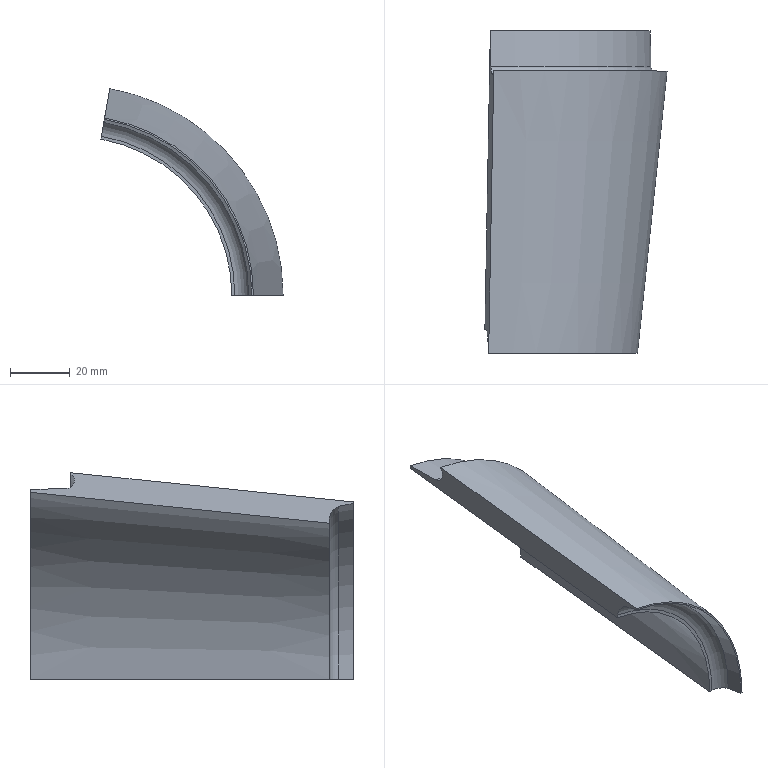Part | STEP file | rubber2 | 1 solid | 12 faces | box 60.803 x 107.596 x 68.922 mm | volume 62752 mm3 | plane 6 | cone 4 | torus 2
STEP:
#1=CARTESIAN_POINT('',(11.001,-64.667,62.388));
#2=VERTEX_POINT('',#1);
#3=CARTESIAN_POINT('',(63.35,-64.667,0.));
#4=VERTEX_POINT('',#3);
#5=CARTESIAN_POINT('',(0.,-64.667,0.));
#6=DIRECTION('',(0.,1.,0.));
#7=DIRECTION('',(0.,0.,1.));
#8=AXIS2_PLACEMENT_3D('',#5,#6,#7);
#9=CIRCLE('',#8,63.35);
#10=EDGE_CURVE('',#2,#4,#9,.T.);
#11=ORIENTED_EDGE('',*,*,#10,.F.);
#12=CARTESIAN_POINT('',(11.174,-64.667,63.372));
#13=VERTEX_POINT('',#12);
#14=CARTESIAN_POINT('',(11.001,-64.667,62.388));
#15=DIRECTION('',(-0.1736,0.,-0.9848));
#16=VECTOR('',#15,1000.);
#17=LINE('',#14,#16);
#18=EDGE_CURVE('',#13,#2,#17,.T.);
#19=ORIENTED_EDGE('',*,*,#18,.F.);
#20=CARTESIAN_POINT('',(64.35,-64.667,0.));
#21=VERTEX_POINT('',#20);
#22=CARTESIAN_POINT('',(0.,-64.667,0.));
#23=DIRECTION('',(0.,1.,0.));
#24=DIRECTION('',(0.,0.,1.));
#25=AXIS2_PLACEMENT_3D('',#22,#23,#24);
#26=CIRCLE('',#25,64.35);
#27=EDGE_CURVE('',#13,#21,#26,.T.);
#28=ORIENTED_EDGE('',*,*,#27,.T.);
#29=CARTESIAN_POINT('',(63.35,-64.667,0.));
#30=DIRECTION('',(-1.,0.,0.));
#31=VECTOR('',#30,1000.);
#32=LINE('',#29,#31);
#33=EDGE_CURVE('',#21,#4,#32,.T.);
#34=ORIENTED_EDGE('',*,*,#33,.T.);
#35=EDGE_LOOP('',(#11,#19,#28,#34));
#36=FACE_OUTER_BOUND('',#35,.T.);
#37=CARTESIAN_POINT('',(11.001,-64.667,62.388));
#38=DIRECTION('',(0.,-1.,0.));
#39=DIRECTION('',(0.,0.,-1.));
#40=AXIS2_PLACEMENT_3D('',#37,#38,#39);
#41=PLANE('',#40);
#42=ADVANCED_FACE('',(#36),#41,.F.);
#43=CARTESIAN_POINT('',(9.183,-164.281,52.077));
#44=VERTEX_POINT('',#43);
#45=CARTESIAN_POINT('',(52.88,-164.281,0.));
#46=VERTEX_POINT('',#45);
#47=CARTESIAN_POINT('',(0.,-164.281,0.));
#48=DIRECTION('',(0.,1.,0.));
#49=DIRECTION('',(0.,0.,1.));
#50=AXIS2_PLACEMENT_3D('',#47,#48,#49);
#51=CIRCLE('',#50,52.88);
#52=EDGE_CURVE('',#44,#46,#51,.T.);
#53=ORIENTED_EDGE('',*,*,#52,.F.);
#54=CARTESIAN_POINT('',(11.001,-64.667,62.388));
#55=DIRECTION('',(-0.01815,-0.9945,-0.1029));
#56=VECTOR('',#55,1000.);
#57=LINE('',#54,#56);
#58=EDGE_CURVE('',#2,#44,#57,.T.);
#59=ORIENTED_EDGE('',*,*,#58,.F.);
#60=ORIENTED_EDGE('',*,*,#10,.T.);
#61=CARTESIAN_POINT('',(63.35,-64.667,0.));
#62=DIRECTION('',(-0.1045,-0.9945,0.));
#63=VECTOR('',#62,1000.);
#64=LINE('',#61,#63);
#65=EDGE_CURVE('',#4,#46,#64,.T.);
#66=ORIENTED_EDGE('',*,*,#65,.T.);
#67=EDGE_LOOP('',(#53,#59,#60,#66));
#68=FACE_OUTER_BOUND('',#67,.T.);
#69=CARTESIAN_POINT('',(0.,-64.667,0.));
#70=DIRECTION('',(0.,1.,0.));
#71=DIRECTION('',(0.,0.,1.));
#72=AXIS2_PLACEMENT_3D('',#69,#70,#71);
#73=CONICAL_SURFACE('',#72,63.35,0.1047);
#74=ADVANCED_FACE('',(#68),#73,.F.);
#75=CARTESIAN_POINT('',(9.356,-164.281,53.062));
#76=VERTEX_POINT('',#75);
#77=CARTESIAN_POINT('',(53.88,-164.281,0.));
#78=VERTEX_POINT('',#77);
#79=CARTESIAN_POINT('',(0.,-164.281,0.));
#80=DIRECTION('',(0.,1.,0.));
#81=DIRECTION('',(0.,0.,1.));
#82=AXIS2_PLACEMENT_3D('',#79,#80,#81);
#83=CIRCLE('',#82,53.88);
#84=EDGE_CURVE('',#76,#78,#83,.T.);
#85=ORIENTED_EDGE('',*,*,#84,.F.);
#86=CARTESIAN_POINT('',(9.183,-164.281,52.077));
#87=DIRECTION('',(0.1736,0.,0.9848));
#88=VECTOR('',#87,1000.);
#89=LINE('',#86,#88);
#90=EDGE_CURVE('',#44,#76,#89,.T.);
#91=ORIENTED_EDGE('',*,*,#90,.F.);
#92=ORIENTED_EDGE('',*,*,#52,.T.);
#93=CARTESIAN_POINT('',(52.88,-164.281,0.));
#94=DIRECTION('',(1.,0.,0.));
#95=VECTOR('',#94,1000.);
#96=LINE('',#93,#95);
#97=EDGE_CURVE('',#46,#78,#96,.T.);
#98=ORIENTED_EDGE('',*,*,#97,.T.);
#99=EDGE_LOOP('',(#85,#91,#92,#98));
#100=FACE_OUTER_BOUND('',#99,.T.);
#101=CARTESIAN_POINT('',(9.183,-164.281,52.077));
#102=DIRECTION('',(0.,1.,0.));
#103=DIRECTION('',(0.,0.,1.));
#104=AXIS2_PLACEMENT_3D('',#101,#102,#103);
#105=PLANE('',#104);
#106=ADVANCED_FACE('',(#100),#105,.F.);
#107=CARTESIAN_POINT('',(10.176,-167.263,57.71));
#108=VERTEX_POINT('',#107);
#109=CARTESIAN_POINT('',(58.6,-167.263,0.));
#110=VERTEX_POINT('',#109);
#111=CARTESIAN_POINT('',(0.,-167.263,0.));
#112=DIRECTION('',(0.,1.,0.));
#113=DIRECTION('',(0.,0.,1.));
#114=AXIS2_PLACEMENT_3D('',#111,#112,#113);
#115=CIRCLE('',#114,58.6);
#116=EDGE_CURVE('',#108,#110,#115,.T.);
#117=ORIENTED_EDGE('',*,*,#116,.F.);
#118=CARTESIAN_POINT('',(9.356,-169.507,53.062));
#119=DIRECTION('',(0.9848,0.,-0.1736));
#120=DIRECTION('',(-0.1736,0.,-0.9848));
#121=AXIS2_PLACEMENT_3D('',#118,#119,#120);
#122=CIRCLE('',#121,5.226);
#123=EDGE_CURVE('',#76,#108,#122,.T.);
#124=ORIENTED_EDGE('',*,*,#123,.F.);
#125=ORIENTED_EDGE('',*,*,#84,.T.);
#126=CARTESIAN_POINT('',(53.88,-169.507,0.));
#127=DIRECTION('',(0.,0.,-1.));
#128=DIRECTION('',(-1.,0.,0.));
#129=AXIS2_PLACEMENT_3D('',#126,#127,#128);
#130=CIRCLE('',#129,5.226);
#131=EDGE_CURVE('',#78,#110,#130,.T.);
#132=ORIENTED_EDGE('',*,*,#131,.T.);
#133=EDGE_LOOP('',(#117,#124,#125,#132));
#134=FACE_OUTER_BOUND('',#133,.T.);
#135=CARTESIAN_POINT('',(0.,-169.507,0.));
#136=DIRECTION('',(0.,1.,0.));
#137=DIRECTION('',(0.,0.,1.));
#138=AXIS2_PLACEMENT_3D('',#135,#136,#137);
#139=TOROIDAL_SURFACE('',#138,53.88,5.226);
#140=ADVANCED_FACE('',(#134),#139,.F.);
#141=CARTESIAN_POINT('',(10.347,-172.263,58.68));
#142=VERTEX_POINT('',#141);
#143=CARTESIAN_POINT('',(59.585,-172.263,0.));
#144=VERTEX_POINT('',#143);
#145=CARTESIAN_POINT('',(0.,-172.263,0.));
#146=DIRECTION('',(0.,1.,0.));
#147=DIRECTION('',(0.,0.,1.));
#148=AXIS2_PLACEMENT_3D('',#145,#146,#147);
#149=CIRCLE('',#148,59.585);
#150=EDGE_CURVE('',#142,#144,#149,.T.);
#151=ORIENTED_EDGE('',*,*,#150,.F.);
#152=CARTESIAN_POINT('',(10.176,-167.263,57.71));
#153=DIRECTION('',(0.03358,-0.9811,0.1904));
#154=VECTOR('',#153,1000.);
#155=LINE('',#152,#154);
#156=EDGE_CURVE('',#108,#142,#155,.T.);
#157=ORIENTED_EDGE('',*,*,#156,.F.);
#158=ORIENTED_EDGE('',*,*,#116,.T.);
#159=CARTESIAN_POINT('',(58.6,-167.263,0.));
#160=DIRECTION('',(0.1934,-0.9811,0.));
#161=VECTOR('',#160,1000.);
#162=LINE('',#159,#161);
#163=EDGE_CURVE('',#110,#144,#162,.T.);
#164=ORIENTED_EDGE('',*,*,#163,.T.);
#165=EDGE_LOOP('',(#151,#157,#158,#164));
#166=FACE_OUTER_BOUND('',#165,.T.);
#167=CARTESIAN_POINT('',(0.,-167.263,0.));
#168=DIRECTION('',(0.,-1.,0.));
#169=DIRECTION('',(0.,0.,-1.));
#170=AXIS2_PLACEMENT_3D('',#167,#168,#169);
#171=CONICAL_SURFACE('',#170,58.6,0.1946);
#172=ADVANCED_FACE('',(#166),#171,.F.);
#173=CARTESIAN_POINT('',(10.434,-172.263,59.172));
#174=VERTEX_POINT('',#173);
#175=CARTESIAN_POINT('',(60.085,-172.263,0.));
#176=VERTEX_POINT('',#175);
#177=CARTESIAN_POINT('',(0.,-172.263,0.));
#178=DIRECTION('',(0.,1.,0.));
#179=DIRECTION('',(0.,0.,1.));
#180=AXIS2_PLACEMENT_3D('',#177,#178,#179);
#181=CIRCLE('',#180,60.085);
#182=EDGE_CURVE('',#174,#176,#181,.T.);
#183=ORIENTED_EDGE('',*,*,#182,.F.);
#184=CARTESIAN_POINT('',(10.434,-172.263,59.172));
#185=DIRECTION('',(0.1736,0.,0.9848));
#186=VECTOR('',#185,1000.);
#187=LINE('',#184,#186);
#188=EDGE_CURVE('',#142,#174,#187,.T.);
#189=ORIENTED_EDGE('',*,*,#188,.F.);
#190=ORIENTED_EDGE('',*,*,#150,.T.);
#191=CARTESIAN_POINT('',(60.085,-172.263,0.));
#192=DIRECTION('',(1.,0.,0.));
#193=VECTOR('',#192,1000.);
#194=LINE('',#191,#193);
#195=EDGE_CURVE('',#144,#176,#194,.T.);
#196=ORIENTED_EDGE('',*,*,#195,.T.);
#197=EDGE_LOOP('',(#183,#189,#190,#196));
#198=FACE_OUTER_BOUND('',#197,.T.);
#199=CARTESIAN_POINT('',(10.434,-172.263,59.172));
#200=DIRECTION('',(0.,1.,0.));
#201=DIRECTION('',(0.,0.,1.));
#202=AXIS2_PLACEMENT_3D('',#199,#200,#201);
#203=PLANE('',#202);
#204=ADVANCED_FACE('',(#198),#203,.F.);
#205=CARTESIAN_POINT('',(12.153,-78.068,68.922));
#206=VERTEX_POINT('',#205);
#207=CARTESIAN_POINT('',(69.986,-78.068,0.));
#208=VERTEX_POINT('',#207);
#209=CARTESIAN_POINT('',(0.,-78.068,0.));
#210=DIRECTION('',(0.,1.,0.));
#211=DIRECTION('',(0.,0.,1.));
#212=AXIS2_PLACEMENT_3D('',#209,#210,#211);
#213=CIRCLE('',#212,69.986);
#214=EDGE_CURVE('',#206,#208,#213,.T.);
#215=ORIENTED_EDGE('',*,*,#214,.F.);
#216=CARTESIAN_POINT('',(12.153,-78.068,68.922));
#217=DIRECTION('',(0.01815,0.9945,0.1029));
#218=VECTOR('',#217,1000.);
#219=LINE('',#216,#218);
#220=EDGE_CURVE('',#174,#206,#219,.T.);
#221=ORIENTED_EDGE('',*,*,#220,.F.);
#222=ORIENTED_EDGE('',*,*,#182,.T.);
#223=CARTESIAN_POINT('',(69.986,-78.068,0.));
#224=DIRECTION('',(0.1045,0.9945,0.));
#225=VECTOR('',#224,1000.);
#226=LINE('',#223,#225);
#227=EDGE_CURVE('',#176,#208,#226,.T.);
#228=ORIENTED_EDGE('',*,*,#227,.T.);
#229=EDGE_LOOP('',(#215,#221,#222,#228));
#230=FACE_OUTER_BOUND('',#229,.T.);
#231=CARTESIAN_POINT('',(0.,-172.263,0.));
#232=DIRECTION('',(0.,1.,0.));
#233=DIRECTION('',(0.,0.,1.));
#234=AXIS2_PLACEMENT_3D('',#231,#232,#233);
#235=CONICAL_SURFACE('',#234,60.085,0.1047);
#236=ADVANCED_FACE('',(#230),#235,.T.);
#237=CARTESIAN_POINT('',(12.066,-78.068,68.43));
#238=VERTEX_POINT('',#237);
#239=CARTESIAN_POINT('',(69.486,-78.068,0.));
#240=VERTEX_POINT('',#239);
#241=CARTESIAN_POINT('',(0.,-78.068,0.));
#242=DIRECTION('',(0.,1.,0.));
#243=DIRECTION('',(0.,0.,1.));
#244=AXIS2_PLACEMENT_3D('',#241,#242,#243);
#245=CIRCLE('',#244,69.486);
#246=EDGE_CURVE('',#238,#240,#245,.T.);
#247=ORIENTED_EDGE('',*,*,#246,.F.);
#248=CARTESIAN_POINT('',(12.153,-78.068,68.922));
#249=DIRECTION('',(-0.1736,0.,-0.9848));
#250=VECTOR('',#249,1000.);
#251=LINE('',#248,#250);
#252=EDGE_CURVE('',#206,#238,#251,.T.);
#253=ORIENTED_EDGE('',*,*,#252,.F.);
#254=ORIENTED_EDGE('',*,*,#214,.T.);
#255=CARTESIAN_POINT('',(69.986,-78.068,0.));
#256=DIRECTION('',(-1.,0.,0.));
#257=VECTOR('',#256,1000.);
#258=LINE('',#255,#257);
#259=EDGE_CURVE('',#208,#240,#258,.T.);
#260=ORIENTED_EDGE('',*,*,#259,.T.);
#261=EDGE_LOOP('',(#247,#253,#254,#260));
#262=FACE_OUTER_BOUND('',#261,.T.);
#263=CARTESIAN_POINT('',(12.153,-78.068,68.922));
#264=DIRECTION('',(0.,-1.,0.));
#265=DIRECTION('',(0.,0.,-1.));
#266=AXIS2_PLACEMENT_3D('',#263,#264,#265);
#267=PLANE('',#266);
#268=ADVANCED_FACE('',(#262),#267,.F.);
#269=CARTESIAN_POINT('',(11.219,-76.601,63.628));
#270=VERTEX_POINT('',#269);
#271=CARTESIAN_POINT('',(64.609,-76.601,0.));
#272=VERTEX_POINT('',#271);
#273=CARTESIAN_POINT('',(0.,-76.601,0.));
#274=DIRECTION('',(0.,1.,0.));
#275=DIRECTION('',(0.,0.,1.));
#276=AXIS2_PLACEMENT_3D('',#273,#274,#275);
#277=CIRCLE('',#276,64.609);
#278=EDGE_CURVE('',#270,#272,#277,.T.);
#279=ORIENTED_EDGE('',*,*,#278,.F.);
#280=CARTESIAN_POINT('',(11.684,-76.542,66.264));
#281=DIRECTION('',(0.9848,0.,-0.1736));
#282=DIRECTION('',(0.1736,0.,0.9848));
#283=AXIS2_PLACEMENT_3D('',#280,#281,#282);
#284=CIRCLE('',#283,2.677);
#285=EDGE_CURVE('',#238,#270,#284,.T.);
#286=ORIENTED_EDGE('',*,*,#285,.F.);
#287=ORIENTED_EDGE('',*,*,#246,.T.);
#288=CARTESIAN_POINT('',(67.286,-76.542,0.));
#289=DIRECTION('',(0.,0.,-1.));
#290=DIRECTION('',(1.,0.,0.));
#291=AXIS2_PLACEMENT_3D('',#288,#289,#290);
#292=CIRCLE('',#291,2.677);
#293=EDGE_CURVE('',#240,#272,#292,.T.);
#294=ORIENTED_EDGE('',*,*,#293,.T.);
#295=EDGE_LOOP('',(#279,#286,#287,#294));
#296=FACE_OUTER_BOUND('',#295,.T.);
#297=CARTESIAN_POINT('',(0.,-76.542,0.));
#298=DIRECTION('',(0.,1.,0.));
#299=DIRECTION('',(0.,0.,1.));
#300=AXIS2_PLACEMENT_3D('',#297,#298,#299);
#301=TOROIDAL_SURFACE('',#300,67.286,2.677);
#302=ADVANCED_FACE('',(#296),#301,.F.);
#303=CARTESIAN_POINT('',(11.174,-64.667,63.372));
#304=DIRECTION('',(-0.003775,0.9998,-0.02141));
#305=VECTOR('',#304,1000.);
#306=LINE('',#303,#305);
#307=EDGE_CURVE('',#270,#13,#306,.T.);
#308=ORIENTED_EDGE('',*,*,#307,.F.);
#309=ORIENTED_EDGE('',*,*,#278,.T.);
#310=CARTESIAN_POINT('',(64.35,-64.667,0.));
#311=DIRECTION('',(-0.02174,0.9998,0.));
#312=VECTOR('',#311,1000.);
#313=LINE('',#310,#312);
#314=EDGE_CURVE('',#272,#21,#313,.T.);
#315=ORIENTED_EDGE('',*,*,#314,.T.);
#316=ORIENTED_EDGE('',*,*,#27,.F.);
#317=EDGE_LOOP('',(#308,#309,#315,#316));
#318=FACE_OUTER_BOUND('',#317,.T.);
#319=CARTESIAN_POINT('',(0.,-76.601,0.));
#320=DIRECTION('',(0.,-1.,0.));
#321=DIRECTION('',(0.,0.,-1.));
#322=AXIS2_PLACEMENT_3D('',#319,#320,#321);
#323=CONICAL_SURFACE('',#322,64.609,0.02174);
#324=ADVANCED_FACE('',(#318),#323,.T.);
#325=ORIENTED_EDGE('',*,*,#18,.T.);
#326=ORIENTED_EDGE('',*,*,#58,.T.);
#327=ORIENTED_EDGE('',*,*,#90,.T.);
#328=ORIENTED_EDGE('',*,*,#123,.T.);
#329=ORIENTED_EDGE('',*,*,#156,.T.);
#330=ORIENTED_EDGE('',*,*,#188,.T.);
#331=ORIENTED_EDGE('',*,*,#220,.T.);
#332=ORIENTED_EDGE('',*,*,#252,.T.);
#333=ORIENTED_EDGE('',*,*,#285,.T.);
#334=ORIENTED_EDGE('',*,*,#307,.T.);
#335=EDGE_LOOP('',(#325,#326,#327,#328,#329,#330,#331,#332,#333,#334));
#336=FACE_OUTER_BOUND('',#335,.T.);
#337=CARTESIAN_POINT('',(11.684,-76.542,66.264));
#338=DIRECTION('',(-0.9848,0.,0.1736));
#339=DIRECTION('',(0.1736,0.,0.9848));
#340=AXIS2_PLACEMENT_3D('',#337,#338,#339);
#341=PLANE('',#340);
#342=ADVANCED_FACE('',(#336),#341,.T.);
#343=ORIENTED_EDGE('',*,*,#33,.F.);
#344=ORIENTED_EDGE('',*,*,#314,.F.);
#345=ORIENTED_EDGE('',*,*,#293,.F.);
#346=ORIENTED_EDGE('',*,*,#259,.F.);
#347=ORIENTED_EDGE('',*,*,#227,.F.);
#348=ORIENTED_EDGE('',*,*,#195,.F.);
#349=ORIENTED_EDGE('',*,*,#163,.F.);
#350=ORIENTED_EDGE('',*,*,#131,.F.);
#351=ORIENTED_EDGE('',*,*,#97,.F.);
#352=ORIENTED_EDGE('',*,*,#65,.F.);
#353=EDGE_LOOP('',(#343,#344,#345,#346,#347,#348,#349,#350,#351,#352));
#354=FACE_OUTER_BOUND('',#353,.T.);
#355=CARTESIAN_POINT('',(67.286,-76.542,0.));
#356=DIRECTION('',(0.,0.,1.));
#357=DIRECTION('',(1.,0.,0.));
#358=AXIS2_PLACEMENT_3D('',#355,#356,#357);
#359=PLANE('',#358);
#360=ADVANCED_FACE('',(#354),#359,.F.);
#361=CLOSED_SHELL('',(#42,#74,#106,#140,#172,#204,#236,#268,#302,#324,#342,#360));
#362=MANIFOLD_SOLID_BREP('',#361);
#363=CARTESIAN_POINT('',(0.,0.,0.));
#364=DIRECTION('',(0.,0.,1.));
#365=DIRECTION('',(1.,0.,0.));
#366=AXIS2_PLACEMENT_3D('',#363,#364,#365);
#367=(LENGTH_UNIT()NAMED_UNIT(*)SI_UNIT(.MILLI.,.METRE.));
#368=UNCERTAINTY_MEASURE_WITH_UNIT(LENGTH_MEASURE(0.00001),#367,'','');
#369=(NAMED_UNIT(*)PLANE_ANGLE_UNIT()SI_UNIT($,.RADIAN.));
#370=(NAMED_UNIT(*)SI_UNIT($,.STERADIAN.)SOLID_ANGLE_UNIT());
#371=(GEOMETRIC_REPRESENTATION_CONTEXT(3)GLOBAL_UNCERTAINTY_ASSIGNED_CONTEXT((#368))GLOBAL_UNIT_ASSIGNED_CONTEXT((#367,#369,#370))REPRESENTATION_CONTEXT('',''));
#372=ADVANCED_BREP_SHAPE_REPRESENTATION('',(#362,#366),#371);